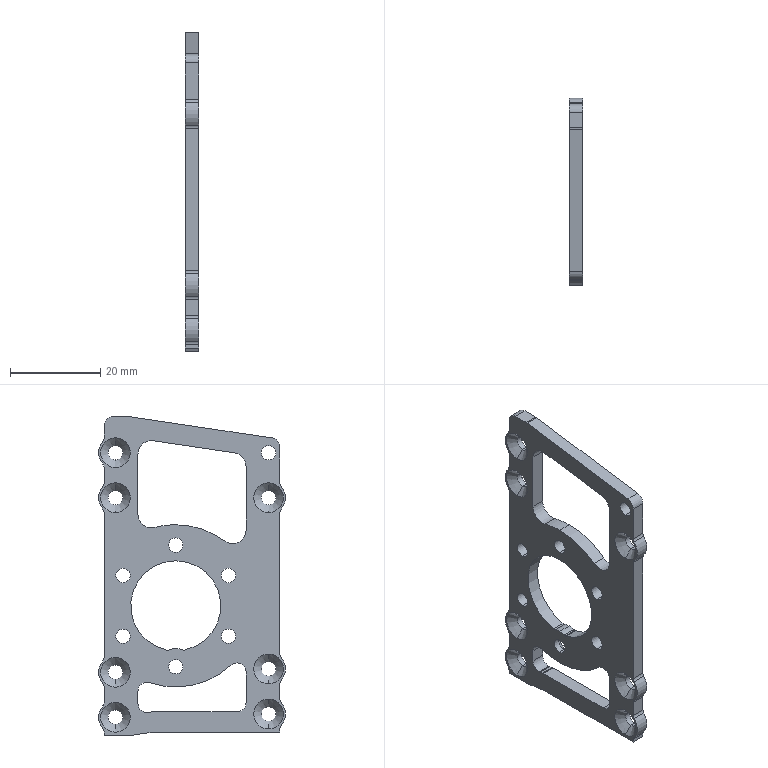Part | SolidWorks | features Fillet 3, HoleWzd 2, ICE 2, Extrusion 1 | 1 solid | 115 faces | box 3 x 41.5 x 70.75 mm | volume 4779 mm3 | cylinder 76 | plane 23 | cone 16 | commonest cylinder face diameters 3.2 x28 2 x17 4 x13 7.5 x7 6 x4 36 x3